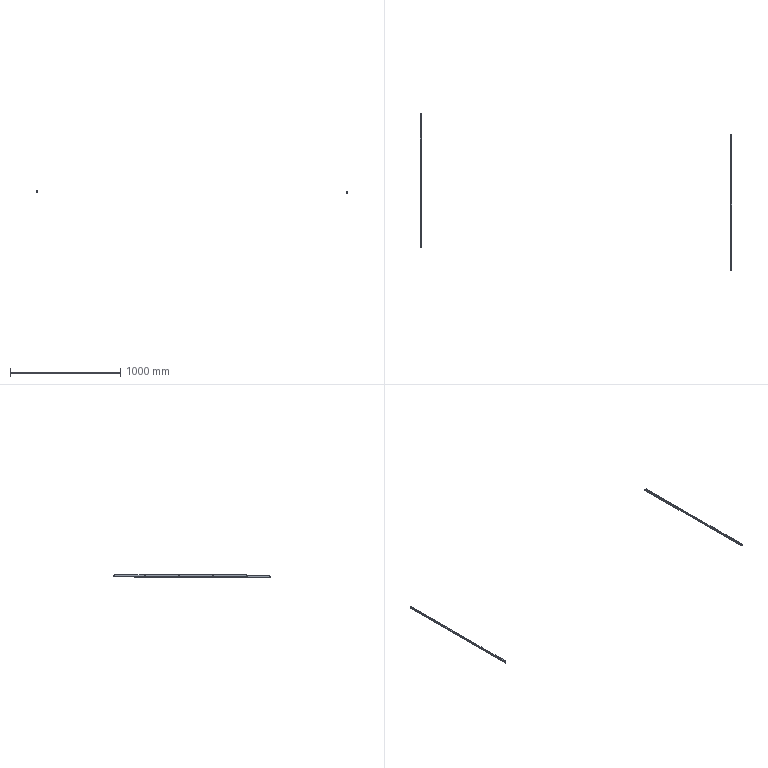NC program | NX | posted with a generic post | part box 2829 x 1430 x 20 mm
Whole program:
N10 G17 G21 G94 G90
(PLANAR_MILL_COPY_COPY_1_COPY_1 , TOOL : D16-48-D16-100-3T-FINISH)
N12 T01 M6
N14 G54
N16 G17 G0 G90 X631. Y0. B0. C0. S4000 M3
N18 G43 Z54. H1
N20 Z5.
N22 G94 G1 Z3. F1000.
N24 X618.
N26 X-618.
N28 X-631.
N30 Z5.
N32 G0 Z54.
N34 X631.
N36 Z4.
N38 G1 Z2.
N40 X618.
N42 X-618.
N44 X-631.
N46 Z4.
N48 G0 Z54.
N50 X631.
N52 Z3.
N54 G1 Z1.
N56 X618.
N58 X-618.
N60 X-631.
N62 Z3.
N64 G0 Z54.
N66 X631.
N68 Z2.1
N70 G1 Z0.1
N72 X618.
N74 X-618.
N76 X-631.
N78 Z2.1
N80 G0 Z54.
(PLANAR_MILL_COPY_COPY_1_COPY_1_COPY , TOOL : D16-48-D16-100-3T-FINISH)
N82 X631.
N84 Z2.
N86 G1 Z0.
N88 X618.
N90 X-618.
N92 X-631.
N94 Z2.
N96 G0 Z54.
N98 M5
(PLANAR_MILL_2_COPY_1_COPY_1 , TOOL : D8-25-D8-60-3T-FINISH)
N100 T03 M6
N102 G54
N104 G17 G0 G90 X-613.9 Y11. B0. C0. S4500 M3
N106 G43 Z50. H3
N108 Z1.
N110 G94 G1 Z-1. F1200.
N112 Y5.
N114 Y-5.
N116 X-612.1
N118 Y5.
N120 Y11.
N122 Z1.
N124 G0 X-613.9 Z0.
N126 G1 Z-2.
N128 Y5.
N130 Y-5.
N132 X-612.1
N134 Y5.
N136 Y11.
N138 Z0.
N140 G0 X-613.9 Z-1.
N142 G1 Z-3.
N144 Y5.
N146 Y-5.
N148 X-612.1
N150 Y5.
N152 Y11.
N154 Z-1.
N156 G0 X-613.9 Z-2.
N158 G1 Z-4.
N160 Y5.
N162 Y-5.
N164 X-612.1
N166 Y5.
N168 Y11.
N170 Z-2.
N172 G0 X-613.9 Z-3.
N174 G1 Z-5.
N176 Y5.
N178 Y-5.
N180 X-612.1
N182 Y5.
N184 Y11.
N186 Z-3.
N188 G0 X-613.9 Z-4.
N190 G1 Z-6.
N192 Y5.
N194 Y-5.
N196 X-612.1
N198 Y5.
N200 Y11.
N202 Z-4.
N204 G0 X-613.9 Z-5.
N206 G1 Z-7.
N208 Y5.
N210 Y-5.
N212 X-612.1
N214 Y5.
N216 Y11.
N218 Z-5.
N220 G0 X-613.9 Z-5.9
N222 G1 Z-7.9
N224 Y5.
N226 Y-5.
N228 X-612.1
N230 Y5.
N232 Y11.
N234 Z-5.9
N236 G0 Z50.
N238 X-317.9
N240 Z1.
N242 G1 Z-1.
N244 Y5.
N246 Y-5.
N248 X-316.1
N250 Y5.
N252 Y11.
N254 Z1.
N256 G0 X-317.9 Z0.
N258 G1 Z-2.
N260 Y5.
N262 Y-5.
N264 X-316.1
N266 Y5.
N268 Y11.
N270 Z0.
N272 G0 X-317.9 Z-1.
N274 G1 Z-3.
N276 Y5.
N278 Y-5.
N280 X-316.1
N282 Y5.
N284 Y11.
N286 Z-1.
N288 G0 X-317.9 Z-2.
N290 G1 Z-4.
N292 Y5.
N294 Y-5.
N296 X-316.1
N298 Y5.
N300 Y11.
N302 Z-2.
N304 G0 X-317.9 Z-3.
N306 G1 Z-5.
N308 Y5.
N310 Y-5.
N312 X-316.1
N314 Y5.
N316 Y11.
N318 Z-3.
N320 G0 X-317.9 Z-4.
N322 G1 Z-6.
N324 Y5.
N326 Y-5.
N328 X-316.1
N330 Y5.
N332 Y11.
N334 Z-4.
N336 G0 X-317.9 Z-5.
N338 G1 Z-7.
N340 Y5.
N342 Y-5.
N344 X-316.1
N346 Y5.
N348 Y11.
N350 Z-5.
N352 G0 X-317.9 Z-5.9
N354 G1 Z-7.9
N356 Y5.
N358 Y-5.
N360 X-316.1
N362 Y5.
N364 Y11.
N366 Z-5.9
N368 G0 Z50.
N370 X-7.9
N372 Z1.
N374 G1 Z-1.
N376 Y5.
N378 Y-5.
N380 X-6.1
N382 Y5.
N384 Y11.
N386 Z1.
N388 G0 X-7.9 Z0.
N390 G1 Z-2.
N392 Y5.
N394 Y-5.
N396 X-6.1
N398 Y5.
N400 Y11.
N402 Z0.
N404 G0 X-7.9 Z-1.
N406 G1 Z-3.
N408 Y5.
N410 Y-5.
N412 X-6.1
N414 Y5.
N416 Y11.
N418 Z-1.
N420 G0 X-7.9 Z-2.
N422 G1 Z-4.
N424 Y5.
N426 Y-5.
N428 X-6.1
N430 Y5.
N432 Y11.
N434 Z-2.
N436 G0 X-7.9 Z-3.
N438 G1 Z-5.
N440 Y5.
N442 Y-5.
N444 X-6.1
N446 Y5.
N448 Y11.
N450 Z-3.
N452 G0 X-7.9 Z-4.
N454 G1 Z-6.
N456 Y5.
N458 Y-5.
N460 X-6.1
N462 Y5.
N464 Y11.
N466 Z-4.
N468 G0 X-7.9 Z-5.
N470 G1 Z-7.
N472 Y5.
N474 Y-5.
N476 X-6.1
N478 Y5.
N480 Y11.
N482 Z-5.
N484 G0 X-7.9 Z-5.9
N486 G1 Z-7.9
N488 Y5.
N490 Y-5.
N492 X-6.1
N494 Y5.
N496 Y11.
N498 Z-5.9
N500 G0 Z50.
N502 X302.1
N504 Z1.
N506 G1 Z-1.
N508 Y5.
N510 Y-5.
N512 X303.9
N514 Y5.
N516 Y11.
N518 Z1.
N520 G0 X302.1 Z0.
N522 G1 Z-2.
N524 Y5.
N526 Y-5.
N528 X303.9
N530 Y5.
N532 Y11.
N534 Z0.
N536 G0 X302.1 Z-1.
N538 G1 Z-3.
N540 Y5.
N542 Y-5.
N544 X303.9
N546 Y5.
N548 Y11.
N550 Z-1.
N552 G0 X302.1 Z-2.
N554 G1 Z-4.
N556 Y5.
N558 Y-5.
N560 X303.9
N562 Y5.
N564 Y11.
N566 Z-2.
N568 G0 X302.1 Z-3.
N570 G1 Z-5.
N572 Y5.
N574 Y-5.
N576 X303.9
N578 Y5.
N580 Y11.
N582 Z-3.
N584 G0 X302.1 Z-4.
N586 G1 Z-6.
N588 Y5.
N590 Y-5.
N592 X303.9
N594 Y5.
N596 Y11.
N598 Z-4.
N600 G0 X302.1 Z-5.
N602 G1 Z-7.
N604 Y5.
N606 Y-5.
N608 X303.9
N610 Y5.
N612 Y11.
N614 Z-5.
N616 G0 X302.1 Z-5.9
N618 G1 Z-7.9
N620 Y5.
N622 Y-5.
N624 X303.9
N626 Y5.
N628 Y11.
N630 Z-5.9
N632 G0 Z50.
N634 X612.1
N636 Z1.
N638 G1 Z-1.
N640 Y5.
N642 Y-5.
N644 X613.9
N646 Y5.
N648 Y11.
N650 Z1.
N652 G0 X612.1 Z0.
N654 G1 Z-2.
N656 Y5.
N658 Y-5.
N660 X613.9
N662 Y5.
N664 Y11.
N666 Z0.
N668 G0 X612.1 Z-1.
N670 G1 Z-3.
N672 Y5.
N674 Y-5.
N676 X613.9
N678 Y5.
N680 Y11.
N682 Z-1.
N684 G0 X612.1 Z-2.
N686 G1 Z-4.
N688 Y5.
N690 Y-5.
N692 X613.9
N694 Y5.
N696 Y11.
N698 Z-2.
N700 G0 X612.1 Z-3.
N702 G1 Z-5.
N704 Y5.
N706 Y-5.
N708 X613.9
N710 Y5.
N712 Y11.
N714 Z-3.
N716 G0 X612.1 Z-4.
N718 G1 Z-6.
N720 Y5.
N722 Y-5.
N724 X613.9
N726 Y5.
N728 Y11.
N730 Z-4.
N732 G0 X612.1 Z-5.
N734 G1 Z-7.
N736 Y5.
N738 Y-5.
N740 X613.9
N742 Y5.
N744 Y11.
N746 Z-5.
N748 G0 X612.1 Z-5.9
N750 G1 Z-7.9
N752 Y5.
N754 Y-5.
N756 X613.9
N758 Y5.
N760 Y11.
N762 Z-5.9
N764 G0 Z50.
(PLANAR_MILL_2_COPY_1_COPY_1_COPY , TOOL : D8-25-D8-60-3T-FINISH)
N766 X-613.965 Y11.197
N768 Z-6.
N770 G1 Z-8. F800.
N772 G41 X-614. Y11. D3
N774 Y5.
N776 Y-5.
N778 X-612.
N780 Y5.
N782 Y11.
N784 G40
N786 X-612.035 Y11.197
N788 Z-6.
N790 G0 Z50.
N792 X-317.965
N794 Z-6.
N796 G1 Z-8.
N798 G41 X-318. Y11.
N800 Y5.
N802 Y-5.
N804 X-316.
N806 Y5.
N808 Y11.
N810 G40
N812 X-316.035 Y11.197
N814 Z-6.
N816 G0 Z50.
N818 X-7.965
N820 Z-6.
N822 G1 Z-8.
N824 G41 X-8. Y11.
N826 Y5.
N828 Y-5.
N830 X-6.
N832 Y5.
N834 Y11.
N836 G40
N838 X-6.035 Y11.197
N840 Z-6.
N842 G0 Z50.
N844 X302.035
N846 Z-6.
N848 G1 Z-8.
N850 G41 X302. Y11.
N852 Y5.
N854 Y-5.
N856 X304.
N858 Y5.
N860 Y11.
N862 G40
N864 X303.965 Y11.197
N866 Z-6.
N868 G0 Z50.
N870 X612.035
N872 Z-6.
N874 G1 Z-8.
N876 G41 X612. Y11.
N878 Y5.
N880 Y-5.
N882 X614.
N884 Y5.
N886 Y11.
N888 G40
N890 X613.965 Y11.197
N892 Z-6.
N894 G0 Z50.
N896 M5
(PLANAR_MILL_3_COPY_COPY , TOOL : 倒角D6-90度)
N898 T04 M6
N900 G54
N902 G17 G0 G90 X456. Y8.5 B0. C0. S3000 M3
N904 G43 Z50. H4
N906 Z0.5
N908 G94 G1 Z-1.5 F1000.
N910 G3 X458. Y6.5 R2.
N912 G1 X608.
N914 G2 X609.5 Y5. R1.5
N916 G1 Y-5.
N918 G2 X608. Y-6.5 R1.5
N920 G1 X308.
N922 G2 X306.5 Y-5. R1.5
N924 G1 Y5.
N926 G2 X308. Y6.5 R1.5
N928 G1 X458.
N930 G3 X460. Y8.5 R2.
N932 G1 Z0.5
N934 G0 Z50.
N936 X146.
N938 Z0.5
N940 G1 Z-1.5
N942 G3 X148. Y6.5 R2.
N944 G1 X298.
N946 G2 X299.5 Y5. R1.5
N948 G1 Y-5.
N950 G2 X298. Y-6.5 R1.5
N952 G1 X-2.
N954 G2 X-3.5 Y-5. R1.5
N956 G1 Y5.
N958 G2 X-2. Y6.5 R1.5
N960 G1 X148.
N962 G3 X150. Y8.5 R2.
N964 G1 Z0.5
N966 G0 Z50.
N968 X-164.
N970 Z0.5
N972 G1 Z-1.5
N974 G3 X-162. Y6.5 R2.
N976 G1 X-12.
N978 G2 X-10.5 Y5. R1.5
N980 G1 Y-5.
N982 G2 X-12. Y-6.5 R1.5
N984 G1 X-312.
N986 G2 X-313.5 Y-5. R1.5
N988 G1 Y5.
N990 G2 X-312. Y6.5 R1.5
N992 G1 X-162.
N994 G3 X-160. Y8.5 R2.
N996 G1 Z0.5
N998 G0 Z50.
N1000 X-467.
N1002 Z0.5
N1004 G1 Z-1.5
N1006 G3 X-465. Y6.5 R2.
N1008 G1 X-322.
N1010 G2 X-320.5 Y5. R1.5
N1012 G1 Y-5.
N1014 G2 X-322. Y-6.5 R1.5
N1016 G1 X-608.
N1018 G2 X-609.5 Y-5. R1.5
N1020 G1 Y5.
N1022 G2 X-608. Y6.5 R1.5
N1024 G1 X-465.
N1026 G3 X-463. Y8.5 R2.
N1028 G1 Z0.5
N1030 G0 Z50.
N1032 M5
N1034 M2